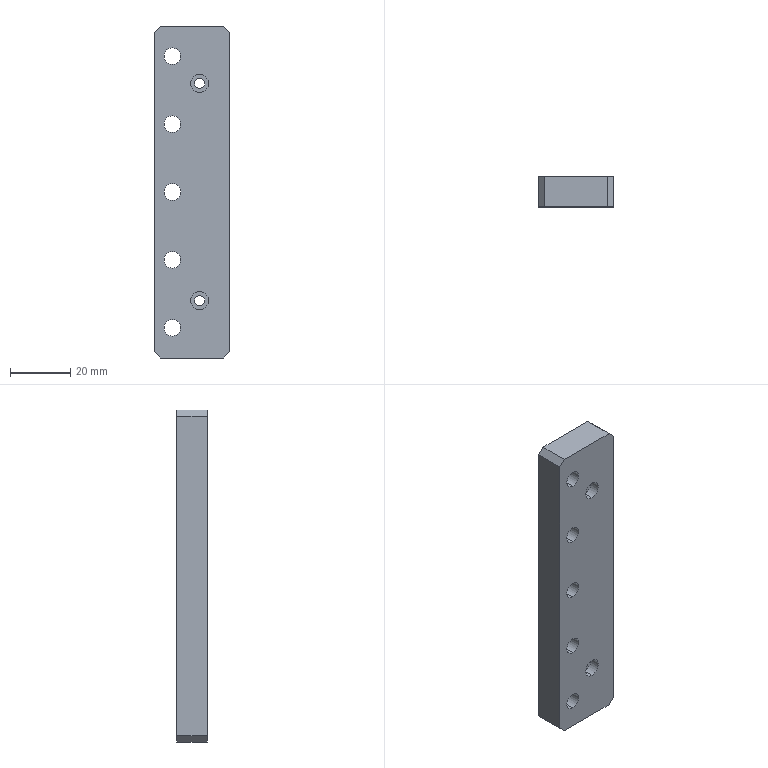Part | SolidWorks | features HoleWzd 3, Chamfer 1, Extrusion 1, ICE 1 | 1 solid | 51 faces | box 25 x 10 x 110 mm | volume 24285 mm3 | cylinder 32 | plane 19 | commonest cylinder face diameters 5.5 x10 10 x10 3.4 x4 5 x4 6 x4
STEP:
#1=CARTESIAN_POINT('',(2.5,6.5,-38.5));
#2=VERTEX_POINT('',#1);
#3=CARTESIAN_POINT('',(2.5,6.5,-33.5));
#4=VERTEX_POINT('',#3);
#5=CARTESIAN_POINT('',(2.5,6.5,-36.));
#6=DIRECTION('',(0.,1.,0.));
#7=DIRECTION('',(0.,0.,1.));
#8=AXIS2_PLACEMENT_3D('',#5,#6,#7);
#9=CIRCLE('',#8,2.5);
#10=EDGE_CURVE('',#2,#4,#9,.T.);
#11=ORIENTED_EDGE('',*,*,#10,.F.);
#12=CARTESIAN_POINT('',(2.5,10.,-38.5));
#13=VERTEX_POINT('',#12);
#14=CARTESIAN_POINT('',(2.5,6.5,-38.5));
#15=DIRECTION('',(0.,1.,0.));
#16=VECTOR('',#15,1000.);
#17=LINE('',#14,#16);
#18=EDGE_CURVE('',#2,#13,#17,.T.);
#19=ORIENTED_EDGE('',*,*,#18,.T.);
#20=CARTESIAN_POINT('',(2.5,10.,-33.5));
#21=VERTEX_POINT('',#20);
#22=CARTESIAN_POINT('',(2.5,10.,-36.));
#23=DIRECTION('',(0.,1.,0.));
#24=DIRECTION('',(0.,0.,1.));
#25=AXIS2_PLACEMENT_3D('',#22,#23,#24);
#26=CIRCLE('',#25,2.5);
#27=EDGE_CURVE('',#13,#21,#26,.T.);
#28=ORIENTED_EDGE('',*,*,#27,.T.);
#29=CARTESIAN_POINT('',(2.5,6.5,-33.5));
#30=DIRECTION('',(0.,1.,0.));
#31=VECTOR('',#30,1000.);
#32=LINE('',#29,#31);
#33=EDGE_CURVE('',#4,#21,#32,.T.);
#34=ORIENTED_EDGE('',*,*,#33,.F.);
#35=EDGE_LOOP('',(#11,#19,#28,#34));
#36=FACE_OUTER_BOUND('',#35,.T.);
#37=CARTESIAN_POINT('',(2.5,6.5,-36.));
#38=DIRECTION('',(0.,1.,0.));
#39=DIRECTION('',(0.,0.,1.));
#40=AXIS2_PLACEMENT_3D('',#37,#38,#39);
#41=CYLINDRICAL_SURFACE('',#40,2.5);
#42=ADVANCED_FACE('',(#36),#41,.F.);
#43=CARTESIAN_POINT('',(2.5,6.5,33.5));
#44=VERTEX_POINT('',#43);
#45=CARTESIAN_POINT('',(2.5,6.5,38.5));
#46=VERTEX_POINT('',#45);
#47=CARTESIAN_POINT('',(2.5,6.5,36.));
#48=DIRECTION('',(0.,1.,0.));
#49=DIRECTION('',(0.,0.,1.));
#50=AXIS2_PLACEMENT_3D('',#47,#48,#49);
#51=CIRCLE('',#50,2.5);
#52=EDGE_CURVE('',#44,#46,#51,.T.);
#53=ORIENTED_EDGE('',*,*,#52,.F.);
#54=CARTESIAN_POINT('',(2.5,10.,33.5));
#55=VERTEX_POINT('',#54);
#56=CARTESIAN_POINT('',(2.5,6.5,33.5));
#57=DIRECTION('',(0.,1.,0.));
#58=VECTOR('',#57,1000.);
#59=LINE('',#56,#58);
#60=EDGE_CURVE('',#44,#55,#59,.T.);
#61=ORIENTED_EDGE('',*,*,#60,.T.);
#62=CARTESIAN_POINT('',(2.5,10.,38.5));
#63=VERTEX_POINT('',#62);
#64=CARTESIAN_POINT('',(2.5,10.,36.));
#65=DIRECTION('',(0.,1.,0.));
#66=DIRECTION('',(0.,0.,1.));
#67=AXIS2_PLACEMENT_3D('',#64,#65,#66);
#68=CIRCLE('',#67,2.5);
#69=EDGE_CURVE('',#55,#63,#68,.T.);
#70=ORIENTED_EDGE('',*,*,#69,.T.);
#71=CARTESIAN_POINT('',(2.5,6.5,38.5));
#72=DIRECTION('',(0.,1.,0.));
#73=VECTOR('',#72,1000.);
#74=LINE('',#71,#73);
#75=EDGE_CURVE('',#46,#63,#74,.T.);
#76=ORIENTED_EDGE('',*,*,#75,.F.);
#77=EDGE_LOOP('',(#53,#61,#70,#76));
#78=FACE_OUTER_BOUND('',#77,.T.);
#79=CARTESIAN_POINT('',(2.5,6.5,36.));
#80=DIRECTION('',(0.,1.,0.));
#81=DIRECTION('',(0.,0.,1.));
#82=AXIS2_PLACEMENT_3D('',#79,#80,#81);
#83=CYLINDRICAL_SURFACE('',#82,2.5);
#84=ADVANCED_FACE('',(#78),#83,.F.);
#85=CARTESIAN_POINT('',(2.5,3.4,39.));
#86=VERTEX_POINT('',#85);
#87=CARTESIAN_POINT('',(2.5,3.4,33.));
#88=VERTEX_POINT('',#87);
#89=CARTESIAN_POINT('',(2.5,3.4,36.));
#90=DIRECTION('',(0.,-1.,0.));
#91=DIRECTION('',(0.,0.,-1.));
#92=AXIS2_PLACEMENT_3D('',#89,#90,#91);
#93=CIRCLE('',#92,3.);
#94=EDGE_CURVE('',#86,#88,#93,.T.);
#95=ORIENTED_EDGE('',*,*,#94,.F.);
#96=CARTESIAN_POINT('',(2.5,0.,39.));
#97=VERTEX_POINT('',#96);
#98=CARTESIAN_POINT('',(2.5,0.,39.));
#99=DIRECTION('',(0.,-1.,0.));
#100=VECTOR('',#99,1000.);
#101=LINE('',#98,#100);
#102=EDGE_CURVE('',#86,#97,#101,.T.);
#103=ORIENTED_EDGE('',*,*,#102,.T.);
#104=CARTESIAN_POINT('',(2.5,0.,33.));
#105=VERTEX_POINT('',#104);
#106=CARTESIAN_POINT('',(2.5,0.,36.));
#107=DIRECTION('',(0.,-1.,0.));
#108=DIRECTION('',(0.,0.,-1.));
#109=AXIS2_PLACEMENT_3D('',#106,#107,#108);
#110=CIRCLE('',#109,3.);
#111=EDGE_CURVE('',#97,#105,#110,.T.);
#112=ORIENTED_EDGE('',*,*,#111,.T.);
#113=CARTESIAN_POINT('',(2.5,0.,33.));
#114=DIRECTION('',(0.,-1.,0.));
#115=VECTOR('',#114,1000.);
#116=LINE('',#113,#115);
#117=EDGE_CURVE('',#88,#105,#116,.T.);
#118=ORIENTED_EDGE('',*,*,#117,.F.);
#119=EDGE_LOOP('',(#95,#103,#112,#118));
#120=FACE_OUTER_BOUND('',#119,.T.);
#121=CARTESIAN_POINT('',(2.5,0.,36.));
#122=DIRECTION('',(0.,-1.,0.));
#123=DIRECTION('',(0.,0.,-1.));
#124=AXIS2_PLACEMENT_3D('',#121,#122,#123);
#125=CYLINDRICAL_SURFACE('',#124,3.);
#126=ADVANCED_FACE('',(#120),#125,.F.);
#127=CARTESIAN_POINT('',(2.5,3.4,-33.));
#128=VERTEX_POINT('',#127);
#129=CARTESIAN_POINT('',(2.5,3.4,-39.));
#130=VERTEX_POINT('',#129);
#131=CARTESIAN_POINT('',(2.5,3.4,-36.));
#132=DIRECTION('',(0.,-1.,0.));
#133=DIRECTION('',(0.,0.,-1.));
#134=AXIS2_PLACEMENT_3D('',#131,#132,#133);
#135=CIRCLE('',#134,3.);
#136=EDGE_CURVE('',#128,#130,#135,.T.);
#137=ORIENTED_EDGE('',*,*,#136,.F.);
#138=CARTESIAN_POINT('',(2.5,0.,-33.));
#139=VERTEX_POINT('',#138);
#140=CARTESIAN_POINT('',(2.5,0.,-33.));
#141=DIRECTION('',(0.,-1.,0.));
#142=VECTOR('',#141,1000.);
#143=LINE('',#140,#142);
#144=EDGE_CURVE('',#128,#139,#143,.T.);
#145=ORIENTED_EDGE('',*,*,#144,.T.);
#146=CARTESIAN_POINT('',(2.5,0.,-39.));
#147=VERTEX_POINT('',#146);
#148=CARTESIAN_POINT('',(2.5,0.,-36.));
#149=DIRECTION('',(0.,-1.,0.));
#150=DIRECTION('',(0.,0.,-1.));
#151=AXIS2_PLACEMENT_3D('',#148,#149,#150);
#152=CIRCLE('',#151,3.);
#153=EDGE_CURVE('',#139,#147,#152,.T.);
#154=ORIENTED_EDGE('',*,*,#153,.T.);
#155=CARTESIAN_POINT('',(2.5,0.,-39.));
#156=DIRECTION('',(0.,-1.,0.));
#157=VECTOR('',#156,1000.);
#158=LINE('',#155,#157);
#159=EDGE_CURVE('',#130,#147,#158,.T.);
#160=ORIENTED_EDGE('',*,*,#159,.F.);
#161=EDGE_LOOP('',(#137,#145,#154,#160));
#162=FACE_OUTER_BOUND('',#161,.T.);
#163=CARTESIAN_POINT('',(2.5,0.,-36.));
#164=DIRECTION('',(0.,-1.,0.));
#165=DIRECTION('',(0.,0.,-1.));
#166=AXIS2_PLACEMENT_3D('',#163,#164,#165);
#167=CYLINDRICAL_SURFACE('',#166,3.);
#168=ADVANCED_FACE('',(#162),#167,.F.);
#169=CARTESIAN_POINT('',(-6.5,4.3,40.));
#170=VERTEX_POINT('',#169);
#171=CARTESIAN_POINT('',(-6.5,4.3,50.));
#172=VERTEX_POINT('',#171);
#173=CARTESIAN_POINT('',(-6.5,4.3,45.));
#174=DIRECTION('',(0.,1.,0.));
#175=DIRECTION('',(0.,0.,1.));
#176=AXIS2_PLACEMENT_3D('',#173,#174,#175);
#177=CIRCLE('',#176,5.);
#178=EDGE_CURVE('',#170,#172,#177,.T.);
#179=ORIENTED_EDGE('',*,*,#178,.F.);
#180=CARTESIAN_POINT('',(-6.5,10.,40.));
#181=VERTEX_POINT('',#180);
#182=CARTESIAN_POINT('',(-6.5,10.,40.));
#183=DIRECTION('',(0.,1.,0.));
#184=VECTOR('',#183,1000.);
#185=LINE('',#182,#184);
#186=EDGE_CURVE('',#170,#181,#185,.T.);
#187=ORIENTED_EDGE('',*,*,#186,.T.);
#188=CARTESIAN_POINT('',(-6.5,10.,50.));
#189=VERTEX_POINT('',#188);
#190=CARTESIAN_POINT('',(-6.5,10.,45.));
#191=DIRECTION('',(0.,1.,0.));
#192=DIRECTION('',(0.,0.,1.));
#193=AXIS2_PLACEMENT_3D('',#190,#191,#192);
#194=CIRCLE('',#193,5.);
#195=EDGE_CURVE('',#181,#189,#194,.T.);
#196=ORIENTED_EDGE('',*,*,#195,.T.);
#197=CARTESIAN_POINT('',(-6.5,10.,50.));
#198=DIRECTION('',(0.,1.,0.));
#199=VECTOR('',#198,1000.);
#200=LINE('',#197,#199);
#201=EDGE_CURVE('',#172,#189,#200,.T.);
#202=ORIENTED_EDGE('',*,*,#201,.F.);
#203=EDGE_LOOP('',(#179,#187,#196,#202));
#204=FACE_OUTER_BOUND('',#203,.T.);
#205=CARTESIAN_POINT('',(-6.5,10.,45.));
#206=DIRECTION('',(0.,1.,0.));
#207=DIRECTION('',(0.,0.,1.));
#208=AXIS2_PLACEMENT_3D('',#205,#206,#207);
#209=CYLINDRICAL_SURFACE('',#208,5.);
#210=ADVANCED_FACE('',(#204),#209,.F.);
#211=CARTESIAN_POINT('',(-6.5,0.,42.25));
#212=VERTEX_POINT('',#211);
#213=CARTESIAN_POINT('',(-6.5,0.,47.75));
#214=VERTEX_POINT('',#213);
#215=CARTESIAN_POINT('',(-6.5,0.,45.));
#216=DIRECTION('',(0.,1.,0.));
#217=DIRECTION('',(0.,0.,1.));
#218=AXIS2_PLACEMENT_3D('',#215,#216,#217);
#219=CIRCLE('',#218,2.75);
#220=EDGE_CURVE('',#212,#214,#219,.T.);
#221=ORIENTED_EDGE('',*,*,#220,.F.);
#222=CARTESIAN_POINT('',(-6.5,4.3,42.25));
#223=VERTEX_POINT('',#222);
#224=CARTESIAN_POINT('',(-6.5,10.,42.25));
#225=DIRECTION('',(0.,1.,0.));
#226=VECTOR('',#225,1000.);
#227=LINE('',#224,#226);
#228=EDGE_CURVE('',#212,#223,#227,.T.);
#229=ORIENTED_EDGE('',*,*,#228,.T.);
#230=CARTESIAN_POINT('',(-6.5,4.3,47.75));
#231=VERTEX_POINT('',#230);
#232=CARTESIAN_POINT('',(-6.5,4.3,45.));
#233=DIRECTION('',(0.,1.,0.));
#234=DIRECTION('',(0.,0.,1.));
#235=AXIS2_PLACEMENT_3D('',#232,#233,#234);
#236=CIRCLE('',#235,2.75);
#237=EDGE_CURVE('',#223,#231,#236,.T.);
#238=ORIENTED_EDGE('',*,*,#237,.T.);
#239=CARTESIAN_POINT('',(-6.5,10.,47.75));
#240=DIRECTION('',(0.,1.,0.));
#241=VECTOR('',#240,1000.);
#242=LINE('',#239,#241);
#243=EDGE_CURVE('',#214,#231,#242,.T.);
#244=ORIENTED_EDGE('',*,*,#243,.F.);
#245=EDGE_LOOP('',(#221,#229,#238,#244));
#246=FACE_OUTER_BOUND('',#245,.T.);
#247=CARTESIAN_POINT('',(-6.5,10.,45.));
#248=DIRECTION('',(0.,1.,0.));
#249=DIRECTION('',(0.,0.,1.));
#250=AXIS2_PLACEMENT_3D('',#247,#248,#249);
#251=CYLINDRICAL_SURFACE('',#250,2.75);
#252=ADVANCED_FACE('',(#246),#251,.F.);
#253=CARTESIAN_POINT('',(-6.5,4.3,-5.));
#254=VERTEX_POINT('',#253);
#255=CARTESIAN_POINT('',(-6.5,4.3,5.));
#256=VERTEX_POINT('',#255);
#257=CARTESIAN_POINT('',(-6.5,4.3,0.));
#258=DIRECTION('',(0.,1.,0.));
#259=DIRECTION('',(0.,0.,1.));
#260=AXIS2_PLACEMENT_3D('',#257,#258,#259);
#261=CIRCLE('',#260,5.);
#262=EDGE_CURVE('',#254,#256,#261,.T.);
#263=ORIENTED_EDGE('',*,*,#262,.F.);
#264=CARTESIAN_POINT('',(-6.5,10.,-5.));
#265=VERTEX_POINT('',#264);
#266=CARTESIAN_POINT('',(-6.5,10.,-5.));
#267=DIRECTION('',(0.,1.,0.));
#268=VECTOR('',#267,1000.);
#269=LINE('',#266,#268);
#270=EDGE_CURVE('',#254,#265,#269,.T.);
#271=ORIENTED_EDGE('',*,*,#270,.T.);
#272=CARTESIAN_POINT('',(-6.5,10.,5.));
#273=VERTEX_POINT('',#272);
#274=CARTESIAN_POINT('',(-6.5,10.,0.));
#275=DIRECTION('',(0.,1.,0.));
#276=DIRECTION('',(0.,0.,1.));
#277=AXIS2_PLACEMENT_3D('',#274,#275,#276);
#278=CIRCLE('',#277,5.);
#279=EDGE_CURVE('',#265,#273,#278,.T.);
#280=ORIENTED_EDGE('',*,*,#279,.T.);
#281=CARTESIAN_POINT('',(-6.5,10.,5.));
#282=DIRECTION('',(0.,1.,0.));
#283=VECTOR('',#282,1000.);
#284=LINE('',#281,#283);
#285=EDGE_CURVE('',#256,#273,#284,.T.);
#286=ORIENTED_EDGE('',*,*,#285,.F.);
#287=EDGE_LOOP('',(#263,#271,#280,#286));
#288=FACE_OUTER_BOUND('',#287,.T.);
#289=CARTESIAN_POINT('',(-6.5,10.,0.));
#290=DIRECTION('',(0.,1.,0.));
#291=DIRECTION('',(0.,0.,1.));
#292=AXIS2_PLACEMENT_3D('',#289,#290,#291);
#293=CYLINDRICAL_SURFACE('',#292,5.);
#294=ADVANCED_FACE('',(#288),#293,.F.);
#295=CARTESIAN_POINT('',(-6.5,0.,-2.75));
#296=VERTEX_POINT('',#295);
#297=CARTESIAN_POINT('',(-6.5,0.,2.75));
#298=VERTEX_POINT('',#297);
#299=CARTESIAN_POINT('',(-6.5,0.,0.));
#300=DIRECTION('',(0.,1.,0.));
#301=DIRECTION('',(0.,0.,1.));
#302=AXIS2_PLACEMENT_3D('',#299,#300,#301);
#303=CIRCLE('',#302,2.75);
#304=EDGE_CURVE('',#296,#298,#303,.T.);
#305=ORIENTED_EDGE('',*,*,#304,.F.);
#306=CARTESIAN_POINT('',(-6.5,4.3,-2.75));
#307=VERTEX_POINT('',#306);
#308=CARTESIAN_POINT('',(-6.5,10.,-2.75));
#309=DIRECTION('',(0.,1.,0.));
#310=VECTOR('',#309,1000.);
#311=LINE('',#308,#310);
#312=EDGE_CURVE('',#296,#307,#311,.T.);
#313=ORIENTED_EDGE('',*,*,#312,.T.);
#314=CARTESIAN_POINT('',(-6.5,4.3,2.75));
#315=VERTEX_POINT('',#314);
#316=CARTESIAN_POINT('',(-6.5,4.3,0.));
#317=DIRECTION('',(0.,1.,0.));
#318=DIRECTION('',(0.,0.,1.));
#319=AXIS2_PLACEMENT_3D('',#316,#317,#318);
#320=CIRCLE('',#319,2.75);
#321=EDGE_CURVE('',#307,#315,#320,.T.);
#322=ORIENTED_EDGE('',*,*,#321,.T.);
#323=CARTESIAN_POINT('',(-6.5,10.,2.75));
#324=DIRECTION('',(0.,1.,0.));
#325=VECTOR('',#324,1000.);
#326=LINE('',#323,#325);
#327=EDGE_CURVE('',#298,#315,#326,.T.);
#328=ORIENTED_EDGE('',*,*,#327,.F.);
#329=EDGE_LOOP('',(#305,#313,#322,#328));
#330=FACE_OUTER_BOUND('',#329,.T.);
#331=CARTESIAN_POINT('',(-6.5,10.,0.));
#332=DIRECTION('',(0.,1.,0.));
#333=DIRECTION('',(0.,0.,1.));
#334=AXIS2_PLACEMENT_3D('',#331,#332,#333);
#335=CYLINDRICAL_SURFACE('',#334,2.75);
#336=ADVANCED_FACE('',(#330),#335,.F.);
#337=CARTESIAN_POINT('',(-6.5,4.3,-50.));
#338=VERTEX_POINT('',#337);
#339=CARTESIAN_POINT('',(-6.5,4.3,-40.));
#340=VERTEX_POINT('',#339);
#341=CARTESIAN_POINT('',(-6.5,4.3,-45.));
#342=DIRECTION('',(0.,1.,0.));
#343=DIRECTION('',(0.,0.,1.));
#344=AXIS2_PLACEMENT_3D('',#341,#342,#343);
#345=CIRCLE('',#344,5.);
#346=EDGE_CURVE('',#338,#340,#345,.T.);
#347=ORIENTED_EDGE('',*,*,#346,.F.);
#348=CARTESIAN_POINT('',(-6.5,10.,-50.));
#349=VERTEX_POINT('',#348);
#350=CARTESIAN_POINT('',(-6.5,10.,-50.));
#351=DIRECTION('',(0.,1.,0.));
#352=VECTOR('',#351,1000.);
#353=LINE('',#350,#352);
#354=EDGE_CURVE('',#338,#349,#353,.T.);
#355=ORIENTED_EDGE('',*,*,#354,.T.);
#356=CARTESIAN_POINT('',(-6.5,10.,-40.));
#357=VERTEX_POINT('',#356);
#358=CARTESIAN_POINT('',(-6.5,10.,-45.));
#359=DIRECTION('',(0.,1.,0.));
#360=DIRECTION('',(0.,0.,1.));
#361=AXIS2_PLACEMENT_3D('',#358,#359,#360);
#362=CIRCLE('',#361,5.);
#363=EDGE_CURVE('',#349,#357,#362,.T.);
#364=ORIENTED_EDGE('',*,*,#363,.T.);
#365=CARTESIAN_POINT('',(-6.5,10.,-40.));
#366=DIRECTION('',(0.,1.,0.));
#367=VECTOR('',#366,1000.);
#368=LINE('',#365,#367);
#369=EDGE_CURVE('',#340,#357,#368,.T.);
#370=ORIENTED_EDGE('',*,*,#369,.F.);
#371=EDGE_LOOP('',(#347,#355,#364,#370));
#372=FACE_OUTER_BOUND('',#371,.T.);
#373=CARTESIAN_POINT('',(-6.5,10.,-45.));
#374=DIRECTION('',(0.,1.,0.));
#375=DIRECTION('',(0.,0.,1.));
#376=AXIS2_PLACEMENT_3D('',#373,#374,#375);
#377=CYLINDRICAL_SURFACE('',#376,5.);
#378=ADVANCED_FACE('',(#372),#377,.F.);
#379=CARTESIAN_POINT('',(-6.5,0.,-47.75));
#380=VERTEX_POINT('',#379);
#381=CARTESIAN_POINT('',(-6.5,0.,-42.25));
#382=VERTEX_POINT('',#381);
#383=CARTESIAN_POINT('',(-6.5,0.,-45.));
#384=DIRECTION('',(0.,1.,0.));
#385=DIRECTION('',(0.,0.,1.));
#386=AXIS2_PLACEMENT_3D('',#383,#384,#385);
#387=CIRCLE('',#386,2.75);
#388=EDGE_CURVE('',#380,#382,#387,.T.);
#389=ORIENTED_EDGE('',*,*,#388,.F.);
#390=CARTESIAN_POINT('',(-6.5,4.3,-47.75));
#391=VERTEX_POINT('',#390);
#392=CARTESIAN_POINT('',(-6.5,10.,-47.75));
#393=DIRECTION('',(0.,1.,0.));
#394=VECTOR('',#393,1000.);
#395=LINE('',#392,#394);
#396=EDGE_CURVE('',#380,#391,#395,.T.);
#397=ORIENTED_EDGE('',*,*,#396,.T.);
#398=CARTESIAN_POINT('',(-6.5,4.3,-42.25));
#399=VERTEX_POINT('',#398);
#400=CARTESIAN_POINT('',(-6.5,4.3,-45.));
#401=DIRECTION('',(0.,1.,0.));
#402=DIRECTION('',(0.,0.,1.));
#403=AXIS2_PLACEMENT_3D('',#400,#401,#402);
#404=CIRCLE('',#403,2.75);
#405=EDGE_CURVE('',#391,#399,#404,.T.);
#406=ORIENTED_EDGE('',*,*,#405,.T.);
#407=CARTESIAN_POINT('',(-6.5,10.,-42.25));
#408=DIRECTION('',(0.,1.,0.));
#409=VECTOR('',#408,1000.);
#410=LINE('',#407,#409);
#411=EDGE_CURVE('',#382,#399,#410,.T.);
#412=ORIENTED_EDGE('',*,*,#411,.F.);
#413=EDGE_LOOP('',(#389,#397,#406,#412));
#414=FACE_OUTER_BOUND('',#413,.T.);
#415=CARTESIAN_POINT('',(-6.5,10.,-45.));
#416=DIRECTION('',(0.,1.,0.));
#417=DIRECTION('',(0.,0.,1.));
#418=AXIS2_PLACEMENT_3D('',#415,#416,#417);
#419=CYLINDRICAL_SURFACE('',#418,2.75);
#420=ADVANCED_FACE('',(#414),#419,.F.);
#421=CARTESIAN_POINT('',(-6.5,4.3,17.5));
#422=VERTEX_POINT('',#421);
#423=CARTESIAN_POINT('',(-6.5,4.3,27.5));
#424=VERTEX_POINT('',#423);
#425=CARTESIAN_POINT('',(-6.5,4.3,22.5));
#426=DIRECTION('',(0.,1.,0.));
#427=DIRECTION('',(0.,0.,1.));
#428=AXIS2_PLACEMENT_3D('',#425,#426,#427);
#429=CIRCLE('',#428,5.);
#430=EDGE_CURVE('',#422,#424,#429,.T.);
#431=ORIENTED_EDGE('',*,*,#430,.F.);
#432=CARTESIAN_POINT('',(-6.5,10.,17.5));
#433=VERTEX_POINT('',#432);
#434=CARTESIAN_POINT('',(-6.5,10.,17.5));
#435=DIRECTION('',(0.,1.,0.));
#436=VECTOR('',#435,1000.);
#437=LINE('',#434,#436);
#438=EDGE_CURVE('',#422,#433,#437,.T.);
#439=ORIENTED_EDGE('',*,*,#438,.T.);
#440=CARTESIAN_POINT('',(-6.5,10.,27.5));
#441=VERTEX_POINT('',#440);
#442=CARTESIAN_POINT('',(-6.5,10.,22.5));
#443=DIRECTION('',(0.,1.,0.));
#444=DIRECTION('',(0.,0.,1.));
#445=AXIS2_PLACEMENT_3D('',#442,#443,#444);
#446=CIRCLE('',#445,5.);
#447=EDGE_CURVE('',#433,#441,#446,.T.);
#448=ORIENTED_EDGE('',*,*,#447,.T.);
#449=CARTESIAN_POINT('',(-6.5,10.,27.5));
#450=DIRECTION('',(0.,1.,0.));
#451=VECTOR('',#450,1000.);
#452=LINE('',#449,#451);
#453=EDGE_CURVE('',#424,#441,#452,.T.);
#454=ORIENTED_EDGE('',*,*,#453,.F.);
#455=EDGE_LOOP('',(#431,#439,#448,#454));
#456=FACE_OUTER_BOUND('',#455,.T.);
#457=CARTESIAN_POINT('',(-6.5,10.,22.5));
#458=DIRECTION('',(0.,1.,0.));
#459=DIRECTION('',(0.,0.,1.));
#460=AXIS2_PLACEMENT_3D('',#457,#458,#459);
#461=CYLINDRICAL_SURFACE('',#460,5.);
#462=ADVANCED_FACE('',(#456),#461,.F.);
#463=CARTESIAN_POINT('',(-6.5,0.,19.75));
#464=VERTEX_POINT('',#463);
#465=CARTESIAN_POINT('',(-6.5,0.,25.25));
#466=VERTEX_POINT('',#465);
#467=CARTESIAN_POINT('',(-6.5,0.,22.5));
#468=DIRECTION('',(0.,1.,0.));
#469=DIRECTION('',(0.,0.,1.));
#470=AXIS2_PLACEMENT_3D('',#467,#468,#469);
#471=CIRCLE('',#470,2.75);
#472=EDGE_CURVE('',#464,#466,#471,.T.);
#473=ORIENTED_EDGE('',*,*,#472,.F.);
#474=CARTESIAN_POINT('',(-6.5,4.3,19.75));
#475=VERTEX_POINT('',#474);
#476=CARTESIAN_POINT('',(-6.5,10.,19.75));
#477=DIRECTION('',(0.,1.,0.));
#478=VECTOR('',#477,1000.);
#479=LINE('',#476,#478);
#480=EDGE_CURVE('',#464,#475,#479,.T.);
#481=ORIENTED_EDGE('',*,*,#480,.T.);
#482=CARTESIAN_POINT('',(-6.5,4.3,25.25));
#483=VERTEX_POINT('',#482);
#484=CARTESIAN_POINT('',(-6.5,4.3,22.5));
#485=DIRECTION('',(0.,1.,0.));
#486=DIRECTION('',(0.,0.,1.));
#487=AXIS2_PLACEMENT_3D('',#484,#485,#486);
#488=CIRCLE('',#487,2.75);
#489=EDGE_CURVE('',#475,#483,#488,.T.);
#490=ORIENTED_EDGE('',*,*,#489,.T.);
#491=CARTESIAN_POINT('',(-6.5,10.,25.25));
#492=DIRECTION('',(0.,1.,0.));
#493=VECTOR('',#492,1000.);
#494=LINE('',#491,#493);
#495=EDGE_CURVE('',#466,#483,#494,.T.);
#496=ORIENTED_EDGE('',*,*,#495,.F.);
#497=EDGE_LOOP('',(#473,#481,#490,#496));
#498=FACE_OUTER_BOUND('',#497,.T.);
#499=CARTESIAN_POINT('',(-6.5,10.,22.5));
#500=DIRECTION('',(0.,1.,0.));
#501=DIRECTION('',(0.,0.,1.));
#502=AXIS2_PLACEMENT_3D('',#499,#500,#501);
#503=CYLINDRICAL_SURFACE('',#502,2.75);
#504=ADVANCED_FACE('',(#498),#503,.F.);
#505=CARTESIAN_POINT('',(-6.5,4.3,-27.5));
#506=VERTEX_POINT('',#505);
#507=CARTESIAN_POINT('',(-6.5,4.3,-17.5));
#508=VERTEX_POINT('',#507);
#509=CARTESIAN_POINT('',(-6.5,4.3,-22.5));
#510=DIRECTION('',(0.,1.,0.));
#511=DIRECTION('',(0.,0.,1.));
#512=AXIS2_PLACEMENT_3D('',#509,#510,#511);
#513=CIRCLE('',#512,5.);
#514=EDGE_CURVE('',#506,#508,#513,.T.);
#515=ORIENTED_EDGE('',*,*,#514,.F.);
#516=CARTESIAN_POINT('',(-6.5,10.,-27.5));
#517=VERTEX_POINT('',#516);
#518=CARTESIAN_POINT('',(-6.5,10.,-27.5));
#519=DIRECTION('',(0.,1.,0.));
#520=VECTOR('',#519,1000.);
#521=LINE('',#518,#520);
#522=EDGE_CURVE('',#506,#517,#521,.T.);
#523=ORIENTED_EDGE('',*,*,#522,.T.);
#524=CARTESIAN_POINT('',(-6.5,10.,-17.5));
#525=VERTEX_POINT('',#524);
#526=CARTESIAN_POINT('',(-6.5,10.,-22.5));
#527=DIRECTION('',(0.,1.,0.));
#528=DIRECTION('',(0.,0.,1.));
#529=AXIS2_PLACEMENT_3D('',#526,#527,#528);
#530=CIRCLE('',#529,5.);
#531=EDGE_CURVE('',#517,#525,#530,.T.);
#532=ORIENTED_EDGE('',*,*,#531,.T.);
#533=CARTESIAN_POINT('',(-6.5,10.,-17.5));
#534=DIRECTION('',(0.,1.,0.));
#535=VECTOR('',#534,1000.);
#536=LINE('',#533,#535);
#537=EDGE_CURVE('',#508,#525,#536,.T.);
#538=ORIENTED_EDGE('',*,*,#537,.F.);
#539=EDGE_LOOP('',(#515,#523,#532,#538));
#540=FACE_OUTER_BOUND('',#539,.T.);
#541=CARTESIAN_POINT('',(-6.5,10.,-22.5));
#542=DIRECTION('',(0.,1.,0.));
#543=DIRECTION('',(0.,0.,1.));
#544=AXIS2_PLACEMENT_3D('',#541,#542,#543);
#545=CYLINDRICAL_SURFACE('',#544,5.);
#546=ADVANCED_FACE('',(#540),#545,.F.);
#547=CARTESIAN_POINT('',(-6.5,0.,-25.25));
#548=VERTEX_POINT('',#547);
#549=CARTESIAN_POINT('',(-6.5,0.,-19.75));
#550=VERTEX_POINT('',#549);
#551=CARTESIAN_POINT('',(-6.5,0.,-22.5));
#552=DIRECTION('',(0.,1.,0.));
#553=DIRECTION('',(0.,0.,1.));
#554=AXIS2_PLACEMENT_3D('',#551,#552,#553);
#555=CIRCLE('',#554,2.75);
#556=EDGE_CURVE('',#548,#550,#555,.T.);
#557=ORIENTED_EDGE('',*,*,#556,.F.);
#558=CARTESIAN_POINT('',(-6.5,4.3,-25.25));
#559=VERTEX_POINT('',#558);
#560=CARTESIAN_POINT('',(-6.5,10.,-25.25));
#561=DIRECTION('',(0.,1.,0.));
#562=VECTOR('',#561,1000.);
#563=LINE('',#560,#562);
#564=EDGE_CURVE('',#548,#559,#563,.T.);
#565=ORIENTED_EDGE('',*,*,#564,.T.);
#566=CARTESIAN_POINT('',(-6.5,4.3,-19.75));
#567=VERTEX_POINT('',#566);
#568=CARTESIAN_POINT('',(-6.5,4.3,-22.5));
#569=DIRECTION('',(0.,1.,0.));
#570=DIRECTION('',(0.,0.,1.));
#571=AXIS2_PLACEMENT_3D('',#568,#569,#570);
#572=CIRCLE('',#571,2.75);
#573=EDGE_CURVE('',#559,#567,#572,.T.);
#574=ORIENTED_EDGE('',*,*,#573,.T.);
#575=CARTESIAN_POINT('',(-6.5,10.,-19.75));
#576=DIRECTION('',(0.,1.,0.));
#577=VECTOR('',#576,1000.);
#578=LINE('',#575,#577);
#579=EDGE_CURVE('',#550,#567,#578,.T.);
#580=ORIENTED_EDGE('',*,*,#579,.F.);
#581=EDGE_LOOP('',(#557,#565,#574,#580));
#582=FACE_OUTER_BOUND('',#581,.T.);
#583=CARTESIAN_POINT('',(-6.5,10.,-22.5));
#584=DIRECTION('',(0.,1.,0.));
#585=DIRECTION('',(0.,0.,1.));
#586=AXIS2_PLACEMENT_3D('',#583,#584,#585);
#587=CYLINDRICAL_SURFACE('',#586,2.75);
#588=ADVANCED_FACE('',(#582),#587,.F.);
#589=CARTESIAN_POINT('',(2.5,6.5,37.7));
#590=VERTEX_POINT('',#589);
#591=CARTESIAN_POINT('',(2.5,6.5,34.3));
#592=VERTEX_POINT('',#591);
#593=CARTESIAN_POINT('',(2.5,6.5,36.));
#594=DIRECTION('',(0.,-1.,0.));
#595=DIRECTION('',(0.,0.,1.));
#596=AXIS2_PLACEMENT_3D('',#593,#594,#595);
#597=CIRCLE('',#596,1.7);
#598=EDGE_CURVE('',#590,#592,#597,.T.);
#599=ORIENTED_EDGE('',*,*,#598,.F.);
#600=CARTESIAN_POINT('',(2.5,3.4,37.7));
#601=VERTEX_POINT('',#600);
#602=CARTESIAN_POINT('',(2.5,0.,37.7));
#603=DIRECTION('',(0.,-1.,0.));
#604=VECTOR('',#603,1000.);
#605=LINE('',#602,#604);
#606=EDGE_CURVE('',#590,#601,#605,.T.);
#607=ORIENTED_EDGE('',*,*,#606,.T.);
#608=CARTESIAN_POINT('',(2.5,3.4,34.3));
#609=VERTEX_POINT('',#608);
#610=CARTESIAN_POINT('',(2.5,3.4,36.));
#611=DIRECTION('',(0.,-1.,0.));
#612=DIRECTION('',(0.,0.,-1.));
#613=AXIS2_PLACEMENT_3D('',#610,#611,#612);
#614=CIRCLE('',#613,1.7);
#615=EDGE_CURVE('',#601,#609,#614,.T.);
#616=ORIENTED_EDGE('',*,*,#615,.T.);
#617=CARTESIAN_POINT('',(2.5,0.,34.3));
#618=DIRECTION('',(0.,-1.,0.));
#619=VECTOR('',#618,1000.);
#620=LINE('',#617,#619);
#621=EDGE_CURVE('',#592,#609,#620,.T.);
#622=ORIENTED_EDGE('',*,*,#621,.F.);
#623=EDGE_LOOP('',(#599,#607,#616,#622));
#624=FACE_OUTER_BOUND('',#623,.T.);
#625=CARTESIAN_POINT('',(2.5,0.,36.));
#626=DIRECTION('',(0.,-1.,0.));
#627=DIRECTION('',(0.,0.,-1.));
#628=AXIS2_PLACEMENT_3D('',#625,#626,#627);
#629=CYLINDRICAL_SURFACE('',#628,1.7);
#630=ADVANCED_FACE('',(#624),#629,.F.);
#631=CARTESIAN_POINT('',(2.5,6.5,-34.3));
#632=VERTEX_POINT('',#631);
#633=CARTESIAN_POINT('',(2.5,6.5,-37.7));
#634=VERTEX_POINT('',#633);
#635=CARTESIAN_POINT('',(2.5,6.5,-36.));
#636=DIRECTION('',(0.,-1.,0.));
#637=DIRECTION('',(0.,0.,1.));
#638=AXIS2_PLACEMENT_3D('',#635,#636,#637);
#639=CIRCLE('',#638,1.7);
#640=EDGE_CURVE('',#632,#634,#639,.T.);
#641=ORIENTED_EDGE('',*,*,#640,.F.);
#642=CARTESIAN_POINT('',(2.5,3.4,-34.3));
#643=VERTEX_POINT('',#642);
#644=CARTESIAN_POINT('',(2.5,0.,-34.3));
#645=DIRECTION('',(0.,-1.,0.));
#646=VECTOR('',#645,1000.);
#647=LINE('',#644,#646);
#648=EDGE_CURVE('',#632,#643,#647,.T.);
#649=ORIENTED_EDGE('',*,*,#648,.T.);
#650=CARTESIAN_POINT('',(2.5,3.4,-37.7));
#651=VERTEX_POINT('',#650);
#652=CARTESIAN_POINT('',(2.5,3.4,-36.));
#653=DIRECTION('',(0.,-1.,0.));
#654=DIRECTION('',(0.,0.,-1.));
#655=AXIS2_PLACEMENT_3D('',#652,#653,#654);
#656=CIRCLE('',#655,1.7);
#657=EDGE_CURVE('',#643,#651,#656,.T.);
#658=ORIENTED_EDGE('',*,*,#657,.T.);
#659=CARTESIAN_POINT('',(2.5,0.,-37.7));
#660=DIRECTION('',(0.,-1.,0.));
#661=VECTOR('',#660,1000.);
#662=LINE('',#659,#661);
#663=EDGE_CURVE('',#634,#651,#662,.T.);
#664=ORIENTED_EDGE('',*,*,#663,.F.);
#665=EDGE_LOOP('',(#641,#649,#658,#664));
#666=FACE_OUTER_BOUND('',#665,.T.);
#667=CARTESIAN_POINT('',(2.5,0.,-36.));
#668=DIRECTION('',(0.,-1.,0.));
#669=DIRECTION('',(0.,0.,-1.));
#670=AXIS2_PLACEMENT_3D('',#667,#668,#669);
#671=CYLINDRICAL_SURFACE('',#670,1.7);
#672=ADVANCED_FACE('',(#666),#671,.F.);
#673=ORIENTED_EDGE('',*,*,#648,.F.);
#674=CARTESIAN_POINT('',(2.5,6.5,-36.));
#675=DIRECTION('',(0.,-1.,0.));
#676=DIRECTION('',(0.,0.,1.));
#677=AXIS2_PLACEMENT_3D('',#674,#675,#676);
#678=CIRCLE('',#677,1.7);
#679=EDGE_CURVE('',#634,#632,#678,.T.);
#680=ORIENTED_EDGE('',*,*,#679,.F.);
#681=ORIENTED_EDGE('',*,*,#663,.T.);
#682=CARTESIAN_POINT('',(2.5,3.4,-36.));
#683=DIRECTION('',(0.,-1.,0.));
#684=DIRECTION('',(0.,0.,-1.));
#685=AXIS2_PLACEMENT_3D('',#682,#683,#684);
#686=CIRCLE('',#685,1.7);
#687=EDGE_CURVE('',#651,#643,#686,.T.);
#688=ORIENTED_EDGE('',*,*,#687,.T.);
#689=EDGE_LOOP('',(#673,#680,#681,#688));
#690=FACE_OUTER_BOUND('',#689,.T.);
#691=CARTESIAN_POINT('',(2.5,0.,-36.));
#692=DIRECTION('',(0.,-1.,0.));
#693=DIRECTION('',(0.,0.,-1.));
#694=AXIS2_PLACEMENT_3D('',#691,#692,#693);
#695=CYLINDRICAL_SURFACE('',#694,1.7);
#696=ADVANCED_FACE('',(#690),#695,.F.);
#697=ORIENTED_EDGE('',*,*,#606,.F.);
#698=CARTESIAN_POINT('',(2.5,6.5,36.));
#699=DIRECTION('',(0.,-1.,0.));
#700=DIRECTION('',(0.,0.,1.));
#701=AXIS2_PLACEMENT_3D('',#698,#699,#700);
#702=CIRCLE('',#701,1.7);
#703=EDGE_CURVE('',#592,#590,#702,.T.);
#704=ORIENTED_EDGE('',*,*,#703,.F.);
#705=ORIENTED_EDGE('',*,*,#621,.T.);
#706=CARTESIAN_POINT('',(2.5,3.4,36.));
#707=DIRECTION('',(0.,-1.,0.));
#708=DIRECTION('',(0.,0.,-1.));
#709=AXIS2_PLACEMENT_3D('',#706,#707,#708);
#710=CIRCLE('',#709,1.7);
#711=EDGE_CURVE('',#609,#601,#710,.T.);
#712=ORIENTED_EDGE('',*,*,#711,.T.);
#713=EDGE_LOOP('',(#697,#704,#705,#712));
#714=FACE_OUTER_BOUND('',#713,.T.);
#715=CARTESIAN_POINT('',(2.5,0.,36.));
#716=DIRECTION('',(0.,-1.,0.));
#717=DIRECTION('',(0.,0.,-1.));
#718=AXIS2_PLACEMENT_3D('',#715,#716,#717);
#719=CYLINDRICAL_SURFACE('',#718,1.7);
#720=ADVANCED_FACE('',(#714),#719,.F.);
#721=CARTESIAN_POINT('',(12.5,0.,53.));
#722=VERTEX_POINT('',#721);
#723=CARTESIAN_POINT('',(12.5,0.,-53.));
#724=VERTEX_POINT('',#723);
#725=CARTESIAN_POINT('',(12.5,0.,-55.));
#726=DIRECTION('',(0.,0.,-1.));
#727=VECTOR('',#726,1000.);
#728=LINE('',#725,#727);
#729=EDGE_CURVE('',#722,#724,#728,.T.);
#730=ORIENTED_EDGE('',*,*,#729,.T.);
#731=CARTESIAN_POINT('',(12.5,10.,-53.));
#732=VERTEX_POINT('',#731);
#733=CARTESIAN_POINT('',(12.5,10.,-53.));
#734=DIRECTION('',(0.,1.,0.));
#735=VECTOR('',#734,1000.);
#736=LINE('',#733,#735);
#737=EDGE_CURVE('',#724,#732,#736,.T.);
#738=ORIENTED_EDGE('',*,*,#737,.T.);
#739=CARTESIAN_POINT('',(12.5,10.,53.));
#740=VERTEX_POINT('',#739);
#741=CARTESIAN_POINT('',(12.5,10.,-55.));
#742=DIRECTION('',(0.,0.,-1.));
#743=VECTOR('',#742,1000.);
#744=LINE('',#741,#743);
#745=EDGE_CURVE('',#740,#732,#744,.T.);
#746=ORIENTED_EDGE('',*,*,#745,.F.);
#747=CARTESIAN_POINT('',(12.5,10.,53.));
#748=DIRECTION('',(0.,-1.,0.));
#749=VECTOR('',#748,1000.);
#750=LINE('',#747,#749);
#751=EDGE_CURVE('',#740,#722,#750,.T.);
#752=ORIENTED_EDGE('',*,*,#751,.T.);
#753=EDGE_LOOP('',(#730,#738,#746,#752));
#754=FACE_OUTER_BOUND('',#753,.T.);
#755=CARTESIAN_POINT('',(12.5,10.,-55.));
#756=DIRECTION('',(-1.,0.,0.));
#757=DIRECTION('',(0.,0.,1.));
#758=AXIS2_PLACEMENT_3D('',#755,#756,#757);
#759=PLANE('',#758);
#760=ADVANCED_FACE('',(#754),#759,.F.);
#761=CARTESIAN_POINT('',(10.5,0.,-55.));
#762=VERTEX_POINT('',#761);
#763=CARTESIAN_POINT('',(-10.5,0.,-55.));
#764=VERTEX_POINT('',#763);
#765=CARTESIAN_POINT('',(-12.5,0.,-55.));
#766=DIRECTION('',(-1.,0.,0.));
#767=VECTOR('',#766,1000.);
#768=LINE('',#765,#767);
#769=EDGE_CURVE('',#762,#764,#768,.T.);
#770=ORIENTED_EDGE('',*,*,#769,.T.);
#771=CARTESIAN_POINT('',(-10.5,10.,-55.));
#772=VERTEX_POINT('',#771);
#773=CARTESIAN_POINT('',(-10.5,10.,-55.));
#774=DIRECTION('',(0.,1.,0.));
#775=VECTOR('',#774,1000.);
#776=LINE('',#773,#775);
#777=EDGE_CURVE('',#764,#772,#776,.T.);
#778=ORIENTED_EDGE('',*,*,#777,.T.);
#779=CARTESIAN_POINT('',(10.5,10.,-55.));
#780=VERTEX_POINT('',#779);
#781=CARTESIAN_POINT('',(-12.5,10.,-55.));
#782=DIRECTION('',(-1.,0.,0.));
#783=VECTOR('',#782,1000.);
#784=LINE('',#781,#783);
#785=EDGE_CURVE('',#780,#772,#784,.T.);
#786=ORIENTED_EDGE('',*,*,#785,.F.);
#787=CARTESIAN_POINT('',(10.5,10.,-55.));
#788=DIRECTION('',(0.,-1.,0.));
#789=VECTOR('',#788,1000.);
#790=LINE('',#787,#789);
#791=EDGE_CURVE('',#780,#762,#790,.T.);
#792=ORIENTED_EDGE('',*,*,#791,.T.);
#793=EDGE_LOOP('',(#770,#778,#786,#792));
#794=FACE_OUTER_BOUND('',#793,.T.);
#795=CARTESIAN_POINT('',(-12.5,10.,-55.));
#796=DIRECTION('',(0.,0.,1.));
#797=DIRECTION('',(1.,0.,0.));
#798=AXIS2_PLACEMENT_3D('',#795,#796,#797);
#799=PLANE('',#798);
#800=ADVANCED_FACE('',(#794),#799,.F.);
#801=CARTESIAN_POINT('',(-12.5,10.,-53.));
#802=VERTEX_POINT('',#801);
#803=CARTESIAN_POINT('',(-12.5,10.,53.));
#804=VERTEX_POINT('',#803);
#805=CARTESIAN_POINT('',(-12.5,10.,-55.));
#806=DIRECTION('',(0.,0.,1.));
#807=VECTOR('',#806,1000.);
#808=LINE('',#805,#807);
#809=EDGE_CURVE('',#802,#804,#808,.T.);
#810=ORIENTED_EDGE('',*,*,#809,.F.);
#811=CARTESIAN_POINT('',(-12.5,0.,-53.));
#812=VERTEX_POINT('',#811);
#813=CARTESIAN_POINT('',(-12.5,10.,-53.));
#814=DIRECTION('',(0.,-1.,0.));
#815=VECTOR('',#814,1000.);
#816=LINE('',#813,#815);
#817=EDGE_CURVE('',#802,#812,#816,.T.);
#818=ORIENTED_EDGE('',*,*,#817,.T.);
#819=CARTESIAN_POINT('',(-12.5,0.,53.));
#820=VERTEX_POINT('',#819);
#821=CARTESIAN_POINT('',(-12.5,0.,-55.));
#822=DIRECTION('',(0.,0.,1.));
#823=VECTOR('',#822,1000.);
#824=LINE('',#821,#823);
#825=EDGE_CURVE('',#812,#820,#824,.T.);
#826=ORIENTED_EDGE('',*,*,#825,.T.);
#827=CARTESIAN_POINT('',(-12.5,10.,53.));
#828=DIRECTION('',(0.,1.,0.));
#829=VECTOR('',#828,1000.);
#830=LINE('',#827,#829);
#831=EDGE_CURVE('',#820,#804,#830,.T.);
#832=ORIENTED_EDGE('',*,*,#831,.T.);
#833=EDGE_LOOP('',(#810,#818,#826,#832));
#834=FACE_OUTER_BOUND('',#833,.T.);
#835=CARTESIAN_POINT('',(-12.5,10.,-55.));
#836=DIRECTION('',(1.,0.,0.));
#837=DIRECTION('',(0.,0.,-1.));
#838=AXIS2_PLACEMENT_3D('',#835,#836,#837);
#839=PLANE('',#838);
#840=ADVANCED_FACE('',(#834),#839,.F.);
#841=CARTESIAN_POINT('',(-10.5,10.,55.));
#842=VERTEX_POINT('',#841);
#843=CARTESIAN_POINT('',(10.5,10.,55.));
#844=VERTEX_POINT('',#843);
#845=CARTESIAN_POINT('',(-12.5,10.,55.));
#846=DIRECTION('',(1.,0.,0.));
#847=VECTOR('',#846,1000.);
#848=LINE('',#845,#847);
#849=EDGE_CURVE('',#842,#844,#848,.T.);
#850=ORIENTED_EDGE('',*,*,#849,.F.);
#851=CARTESIAN_POINT('',(-10.5,0.,55.));
#852=VERTEX_POINT('',#851);
#853=CARTESIAN_POINT('',(-10.5,10.,55.));
#854=DIRECTION('',(0.,-1.,0.));
#855=VECTOR('',#854,1000.);
#856=LINE('',#853,#855);
#857=EDGE_CURVE('',#842,#852,#856,.T.);
#858=ORIENTED_EDGE('',*,*,#857,.T.);
#859=CARTESIAN_POINT('',(10.5,0.,55.));
#860=VERTEX_POINT('',#859);
#861=CARTESIAN_POINT('',(-12.5,0.,55.));
#862=DIRECTION('',(1.,0.,0.));
#863=VECTOR('',#862,1000.);
#864=LINE('',#861,#863);
#865=EDGE_CURVE('',#852,#860,#864,.T.);
#866=ORIENTED_EDGE('',*,*,#865,.T.);
#867=CARTESIAN_POINT('',(10.5,10.,55.));
#868=DIRECTION('',(0.,1.,0.));
#869=VECTOR('',#868,1000.);
#870=LINE('',#867,#869);
#871=EDGE_CURVE('',#860,#844,#870,.T.);
#872=ORIENTED_EDGE('',*,*,#871,.T.);
#873=EDGE_LOOP('',(#850,#858,#866,#872));
#874=FACE_OUTER_BOUND('',#873,.T.);
#875=CARTESIAN_POINT('',(-12.5,10.,55.));
#876=DIRECTION('',(0.,0.,-1.));
#877=DIRECTION('',(-1.,0.,0.));
#878=AXIS2_PLACEMENT_3D('',#875,#876,#877);
#879=PLANE('',#878);
#880=ADVANCED_FACE('',(#874),#879,.F.);
#881=CARTESIAN_POINT('',(2.5,10.,36.));
#882=DIRECTION('',(0.,1.,0.));
#883=DIRECTION('',(0.,0.,1.));
#884=AXIS2_PLACEMENT_3D('',#881,#882,#883);
#885=CIRCLE('',#884,2.5);
#886=EDGE_CURVE('',#63,#55,#885,.T.);
#887=ORIENTED_EDGE('',*,*,#886,.F.);
#888=ORIENTED_EDGE('',*,*,#69,.F.);
#889=EDGE_LOOP('',(#887,#888));
#890=FACE_BOUND('',#889,.T.);
#891=CARTESIAN_POINT('',(2.5,10.,-36.));
#892=DIRECTION('',(0.,1.,0.));
#893=DIRECTION('',(0.,0.,1.));
#894=AXIS2_PLACEMENT_3D('',#891,#892,#893);
#895=CIRCLE('',#894,2.5);
#896=EDGE_CURVE('',#21,#13,#895,.T.);
#897=ORIENTED_EDGE('',*,*,#896,.F.);
#898=ORIENTED_EDGE('',*,*,#27,.F.);
#899=EDGE_LOOP('',(#897,#898));
#900=FACE_BOUND('',#899,.T.);
#901=CARTESIAN_POINT('',(-6.5,10.,45.));
#902=DIRECTION('',(0.,1.,0.));
#903=DIRECTION('',(0.,0.,1.));
#904=AXIS2_PLACEMENT_3D('',#901,#902,#903);
#905=CIRCLE('',#904,5.);
#906=EDGE_CURVE('',#189,#181,#905,.T.);
#907=ORIENTED_EDGE('',*,*,#906,.F.);
#908=ORIENTED_EDGE('',*,*,#195,.F.);
#909=EDGE_LOOP('',(#907,#908));
#910=FACE_BOUND('',#909,.T.);
#911=CARTESIAN_POINT('',(-6.5,10.,0.));
#912=DIRECTION('',(0.,1.,0.));
#913=DIRECTION('',(0.,0.,1.));
#914=AXIS2_PLACEMENT_3D('',#911,#912,#913);
#915=CIRCLE('',#914,5.);
#916=EDGE_CURVE('',#273,#265,#915,.T.);
#917=ORIENTED_EDGE('',*,*,#916,.F.);
#918=ORIENTED_EDGE('',*,*,#279,.F.);
#919=EDGE_LOOP('',(#917,#918));
#920=FACE_BOUND('',#919,.T.);
#921=CARTESIAN_POINT('',(-6.5,10.,-45.));
#922=DIRECTION('',(0.,1.,0.));
#923=DIRECTION('',(0.,0.,1.));
#924=AXIS2_PLACEMENT_3D('',#921,#922,#923);
#925=CIRCLE('',#924,5.);
#926=EDGE_CURVE('',#357,#349,#925,.T.);
#927=ORIENTED_EDGE('',*,*,#926,.F.);
#928=ORIENTED_EDGE('',*,*,#363,.F.);
#929=EDGE_LOOP('',(#927,#928));
#930=FACE_BOUND('',#929,.T.);
#931=CARTESIAN_POINT('',(-6.5,10.,22.5));
#932=DIRECTION('',(0.,1.,0.));
#933=DIRECTION('',(0.,0.,1.));
#934=AXIS2_PLACEMENT_3D('',#931,#932,#933);
#935=CIRCLE('',#934,5.);
#936=EDGE_CURVE('',#441,#433,#935,.T.);
#937=ORIENTED_EDGE('',*,*,#936,.F.);
#938=ORIENTED_EDGE('',*,*,#447,.F.);
#939=EDGE_LOOP('',(#937,#938));
#940=FACE_BOUND('',#939,.T.);
#941=CARTESIAN_POINT('',(-6.5,10.,-22.5));
#942=DIRECTION('',(0.,1.,0.));
#943=DIRECTION('',(0.,0.,1.));
#944=AXIS2_PLACEMENT_3D('',#941,#942,#943);
#945=CIRCLE('',#944,5.);
#946=EDGE_CURVE('',#525,#517,#945,.T.);
#947=ORIENTED_EDGE('',*,*,#946,.F.);
#948=ORIENTED_EDGE('',*,*,#531,.F.);
#949=EDGE_LOOP('',(#947,#948));
#950=FACE_BOUND('',#949,.T.);
#951=ORIENTED_EDGE('',*,*,#785,.T.);
#952=CARTESIAN_POINT('',(-32.75,10.,-32.75));
#953=DIRECTION('',(-0.7071,0.,0.7071));
#954=VECTOR('',#953,1000.);
#955=LINE('',#952,#954);
#956=EDGE_CURVE('',#772,#802,#955,.T.);
#957=ORIENTED_EDGE('',*,*,#956,.T.);
#958=ORIENTED_EDGE('',*,*,#809,.T.);
#959=CARTESIAN_POINT('',(-32.75,10.,32.75));
#960=DIRECTION('',(0.7071,0.,0.7071));
#961=VECTOR('',#960,1000.);
#962=LINE('',#959,#961);
#963=EDGE_CURVE('',#804,#842,#962,.T.);
#964=ORIENTED_EDGE('',*,*,#963,.T.);
#965=ORIENTED_EDGE('',*,*,#849,.T.);
#966=CARTESIAN_POINT('',(32.75,10.,32.75));
#967=DIRECTION('',(0.7071,0.,-0.7071));
#968=VECTOR('',#967,1000.);
#969=LINE('',#966,#968);
#970=EDGE_CURVE('',#844,#740,#969,.T.);
#971=ORIENTED_EDGE('',*,*,#970,.T.);
#972=ORIENTED_EDGE('',*,*,#745,.T.);
#973=CARTESIAN_POINT('',(32.75,10.,-32.75));
#974=DIRECTION('',(-0.7071,0.,-0.7071));
#975=VECTOR('',#974,1000.);
#976=LINE('',#973,#975);
#977=EDGE_CURVE('',#732,#780,#976,.T.);
#978=ORIENTED_EDGE('',*,*,#977,.T.);
#979=EDGE_LOOP('',(#951,#957,#958,#964,#965,#971,#972,#978));
#980=FACE_OUTER_BOUND('',#979,.T.);
#981=CARTESIAN_POINT('',(0.,10.,0.));
#982=DIRECTION('',(0.,1.,0.));
#983=DIRECTION('',(0.,0.,1.));
#984=AXIS2_PLACEMENT_3D('',#981,#982,#983);
#985=PLANE('',#984);
#986=ADVANCED_FACE('',(#890,#900,#910,#920,#930,#940,#950,#980),#985,.T.);
#987=CARTESIAN_POINT('',(2.5,0.,36.));
#988=DIRECTION('',(0.,-1.,0.));
#989=DIRECTION('',(0.,0.,-1.));
#990=AXIS2_PLACEMENT_3D('',#987,#988,#989);
#991=CIRCLE('',#990,3.);
#992=EDGE_CURVE('',#105,#97,#991,.T.);
#993=ORIENTED_EDGE('',*,*,#992,.F.);
#994=ORIENTED_EDGE('',*,*,#111,.F.);
#995=EDGE_LOOP('',(#993,#994));
#996=FACE_BOUND('',#995,.T.);
#997=CARTESIAN_POINT('',(2.5,0.,-36.));
#998=DIRECTION('',(0.,-1.,0.));
#999=DIRECTION('',(0.,0.,-1.));
#1000=AXIS2_PLACEMENT_3D('',#997,#998,#999);
#1001=CIRCLE('',#1000,3.);
#1002=EDGE_CURVE('',#147,#139,#1001,.T.);
#1003=ORIENTED_EDGE('',*,*,#1002,.F.);
#1004=ORIENTED_EDGE('',*,*,#153,.F.);
#1005=EDGE_LOOP('',(#1003,#1004));
#1006=FACE_BOUND('',#1005,.T.);
#1007=CARTESIAN_POINT('',(-6.5,0.,45.));
#1008=DIRECTION('',(0.,1.,0.));
#1009=DIRECTION('',(0.,0.,1.));
#1010=AXIS2_PLACEMENT_3D('',#1007,#1008,#1009);
#1011=CIRCLE('',#1010,2.75);
#1012=EDGE_CURVE('',#214,#212,#1011,.T.);
#1013=ORIENTED_EDGE('',*,*,#1012,.T.);
#1014=ORIENTED_EDGE('',*,*,#220,.T.);
#1015=EDGE_LOOP('',(#1013,#1014));
#1016=FACE_BOUND('',#1015,.T.);
#1017=CARTESIAN_POINT('',(-6.5,0.,0.));
#1018=DIRECTION('',(0.,1.,0.));
#1019=DIRECTION('',(0.,0.,1.));
#1020=AXIS2_PLACEMENT_3D('',#1017,#1018,#1019);
#1021=CIRCLE('',#1020,2.75);
#1022=EDGE_CURVE('',#298,#296,#1021,.T.);
#1023=ORIENTED_EDGE('',*,*,#1022,.T.);
#1024=ORIENTED_EDGE('',*,*,#304,.T.);
#1025=EDGE_LOOP('',(#1023,#1024));
#1026=FACE_BOUND('',#1025,.T.);
#1027=CARTESIAN_POINT('',(-6.5,0.,-45.));
#1028=DIRECTION('',(0.,1.,0.));
#1029=DIRECTION('',(0.,0.,1.));
#1030=AXIS2_PLACEMENT_3D('',#1027,#1028,#1029);
#1031=CIRCLE('',#1030,2.75);
#1032=EDGE_CURVE('',#382,#380,#1031,.T.);
#1033=ORIENTED_EDGE('',*,*,#1032,.T.);
#1034=ORIENTED_EDGE('',*,*,#388,.T.);
#1035=EDGE_LOOP('',(#1033,#1034));
#1036=FACE_BOUND('',#1035,.T.);
#1037=CARTESIAN_POINT('',(-6.5,0.,22.5));
#1038=DIRECTION('',(0.,1.,0.));
#1039=DIRECTION('',(0.,0.,1.));
#1040=AXIS2_PLACEMENT_3D('',#1037,#1038,#1039);
#1041=CIRCLE('',#1040,2.75);
#1042=EDGE_CURVE('',#466,#464,#1041,.T.);
#1043=ORIENTED_EDGE('',*,*,#1042,.T.);
#1044=ORIENTED_EDGE('',*,*,#472,.T.);
#1045=EDGE_LOOP('',(#1043,#1044));
#1046=FACE_BOUND('',#1045,.T.);
#1047=CARTESIAN_POINT('',(-6.5,0.,-22.5));
#1048=DIRECTION('',(0.,1.,0.));
#1049=DIRECTION('',(0.,0.,1.));
#1050=AXIS2_PLACEMENT_3D('',#1047,#1048,#1049);
#1051=CIRCLE('',#1050,2.75);
#1052=EDGE_CURVE('',#550,#548,#1051,.T.);
#1053=ORIENTED_EDGE('',*,*,#1052,.T.);
#1054=ORIENTED_EDGE('',*,*,#556,.T.);
#1055=EDGE_LOOP('',(#1053,#1054));
#1056=FACE_BOUND('',#1055,.T.);
#1057=ORIENTED_EDGE('',*,*,#825,.F.);
#1058=CARTESIAN_POINT('',(-12.5,0.,-53.));
#1059=DIRECTION('',(0.7071,0.,-0.7071));
#1060=VECTOR('',#1059,1000.);
#1061=LINE('',#1058,#1060);
#1062=EDGE_CURVE('',#812,#764,#1061,.T.);
#1063=ORIENTED_EDGE('',*,*,#1062,.T.);
#1064=ORIENTED_EDGE('',*,*,#769,.F.);
#1065=CARTESIAN_POINT('',(10.5,0.,-55.));
#1066=DIRECTION('',(0.7071,0.,0.7071));
#1067=VECTOR('',#1066,1000.);
#1068=LINE('',#1065,#1067);
#1069=EDGE_CURVE('',#762,#724,#1068,.T.);
#1070=ORIENTED_EDGE('',*,*,#1069,.T.);
#1071=ORIENTED_EDGE('',*,*,#729,.F.);
#1072=CARTESIAN_POINT('',(12.5,0.,53.));
#1073=DIRECTION('',(-0.7071,0.,0.7071));
#1074=VECTOR('',#1073,1000.);
#1075=LINE('',#1072,#1074);
#1076=EDGE_CURVE('',#722,#860,#1075,.T.);
#1077=ORIENTED_EDGE('',*,*,#1076,.T.);
#1078=ORIENTED_EDGE('',*,*,#865,.F.);
#1079=CARTESIAN_POINT('',(-10.5,0.,55.));
#1080=DIRECTION('',(-0.7071,0.,-0.7071));
#1081=VECTOR('',#1080,1000.);
#1082=LINE('',#1079,#1081);
#1083=EDGE_CURVE('',#852,#820,#1082,.T.);
#1084=ORIENTED_EDGE('',*,*,#1083,.T.);
#1085=EDGE_LOOP('',(#1057,#1063,#1064,#1070,#1071,#1077,#1078,#1084));
#1086=FACE_OUTER_BOUND('',#1085,.T.);
#1087=CARTESIAN_POINT('',(0.,0.,0.));
#1088=DIRECTION('',(0.,1.,0.));
#1089=DIRECTION('',(0.,0.,1.));
#1090=AXIS2_PLACEMENT_3D('',#1087,#1088,#1089);
#1091=PLANE('',#1090);
#1092=ADVANCED_FACE('',(#996,#1006,#1016,#1026,#1036,#1046,#1056,#1086),#1091,.F.);
#1093=ORIENTED_EDGE('',*,*,#956,.F.);
#1094=ORIENTED_EDGE('',*,*,#777,.F.);
#1095=ORIENTED_EDGE('',*,*,#1062,.F.);
#1096=ORIENTED_EDGE('',*,*,#817,.F.);
#1097=EDGE_LOOP('',(#1093,#1094,#1095,#1096));
#1098=FACE_OUTER_BOUND('',#1097,.T.);
#1099=CARTESIAN_POINT('',(-12.5,10.,-53.));
#1100=DIRECTION('',(0.7071,0.,0.7071));
#1101=DIRECTION('',(0.,-1.,0.));
#1102=AXIS2_PLACEMENT_3D('',#1099,#1100,#1101);
#1103=PLANE('',#1102);
#1104=ADVANCED_FACE('',(#1098),#1103,.F.);
#1105=ORIENTED_EDGE('',*,*,#977,.F.);
#1106=ORIENTED_EDGE('',*,*,#737,.F.);
#1107=ORIENTED_EDGE('',*,*,#1069,.F.);
#1108=ORIENTED_EDGE('',*,*,#791,.F.);
#1109=EDGE_LOOP('',(#1105,#1106,#1107,#1108));
#1110=FACE_OUTER_BOUND('',#1109,.T.);
#1111=CARTESIAN_POINT('',(10.5,10.,-55.));
#1112=DIRECTION('',(-0.7071,0.,0.7071));
#1113=DIRECTION('',(0.,-1.,0.));
#1114=AXIS2_PLACEMENT_3D('',#1111,#1112,#1113);
#1115=PLANE('',#1114);
#1116=ADVANCED_FACE('',(#1110),#1115,.F.);
#1117=ORIENTED_EDGE('',*,*,#963,.F.);
#1118=ORIENTED_EDGE('',*,*,#831,.F.);
#1119=ORIENTED_EDGE('',*,*,#1083,.F.);
#1120=ORIENTED_EDGE('',*,*,#857,.F.);
#1121=EDGE_LOOP('',(#1117,#1118,#1119,#1120));
#1122=FACE_OUTER_BOUND('',#1121,.T.);
#1123=CARTESIAN_POINT('',(-10.5,10.,55.));
#1124=DIRECTION('',(0.7071,0.,-0.7071));
#1125=DIRECTION('',(0.,-1.,0.));
#1126=AXIS2_PLACEMENT_3D('',#1123,#1124,#1125);
#1127=PLANE('',#1126);
#1128=ADVANCED_FACE('',(#1122),#1127,.F.);
#1129=ORIENTED_EDGE('',*,*,#970,.F.);
#1130=ORIENTED_EDGE('',*,*,#871,.F.);
#1131=ORIENTED_EDGE('',*,*,#1076,.F.);
#1132=ORIENTED_EDGE('',*,*,#751,.F.);
#1133=EDGE_LOOP('',(#1129,#1130,#1131,#1132));
#1134=FACE_OUTER_BOUND('',#1133,.T.);
#1135=CARTESIAN_POINT('',(12.5,10.,53.));
#1136=DIRECTION('',(-0.7071,0.,-0.7071));
#1137=DIRECTION('',(0.,-1.,0.));
#1138=AXIS2_PLACEMENT_3D('',#1135,#1136,#1137);
#1139=PLANE('',#1138);
#1140=ADVANCED_FACE('',(#1134),#1139,.F.);
#1141=ORIENTED_EDGE('',*,*,#564,.F.);
#1142=ORIENTED_EDGE('',*,*,#1052,.F.);
#1143=ORIENTED_EDGE('',*,*,#579,.T.);
#1144=CARTESIAN_POINT('',(-6.5,4.3,-22.5));
#1145=DIRECTION('',(0.,1.,0.));
#1146=DIRECTION('',(0.,0.,1.));
#1147=AXIS2_PLACEMENT_3D('',#1144,#1145,#1146);
#1148=CIRCLE('',#1147,2.75);
#1149=EDGE_CURVE('',#567,#559,#1148,.T.);
#1150=ORIENTED_EDGE('',*,*,#1149,.T.);
#1151=EDGE_LOOP('',(#1141,#1142,#1143,#1150));
#1152=FACE_OUTER_BOUND('',#1151,.T.);
#1153=CARTESIAN_POINT('',(-6.5,10.,-22.5));
#1154=DIRECTION('',(0.,1.,0.));
#1155=DIRECTION('',(0.,0.,1.));
#1156=AXIS2_PLACEMENT_3D('',#1153,#1154,#1155);
#1157=CYLINDRICAL_SURFACE('',#1156,2.75);
#1158=ADVANCED_FACE('',(#1152),#1157,.F.);
#1159=ORIENTED_EDGE('',*,*,#1149,.F.);
#1160=ORIENTED_EDGE('',*,*,#573,.F.);
#1161=EDGE_LOOP('',(#1159,#1160));
#1162=FACE_BOUND('',#1161,.T.);
#1163=CARTESIAN_POINT('',(-6.5,4.3,-22.5));
#1164=DIRECTION('',(0.,1.,0.));
#1165=DIRECTION('',(0.,0.,1.));
#1166=AXIS2_PLACEMENT_3D('',#1163,#1164,#1165);
#1167=CIRCLE('',#1166,5.);
#1168=EDGE_CURVE('',#508,#506,#1167,.T.);
#1169=ORIENTED_EDGE('',*,*,#1168,.T.);
#1170=ORIENTED_EDGE('',*,*,#514,.T.);
#1171=EDGE_LOOP('',(#1169,#1170));
#1172=FACE_OUTER_BOUND('',#1171,.T.);
#1173=CARTESIAN_POINT('',(-3.75,4.3,-22.5));
#1174=DIRECTION('',(0.,-1.,0.));
#1175=DIRECTION('',(0.,0.,-1.));
#1176=AXIS2_PLACEMENT_3D('',#1173,#1174,#1175);
#1177=PLANE('',#1176);
#1178=ADVANCED_FACE('',(#1162,#1172),#1177,.F.);
#1179=ORIENTED_EDGE('',*,*,#522,.F.);
#1180=ORIENTED_EDGE('',*,*,#1168,.F.);
#1181=ORIENTED_EDGE('',*,*,#537,.T.);
#1182=ORIENTED_EDGE('',*,*,#946,.T.);
#1183=EDGE_LOOP('',(#1179,#1180,#1181,#1182));
#1184=FACE_OUTER_BOUND('',#1183,.T.);
#1185=CARTESIAN_POINT('',(-6.5,10.,-22.5));
#1186=DIRECTION('',(0.,1.,0.));
#1187=DIRECTION('',(0.,0.,1.));
#1188=AXIS2_PLACEMENT_3D('',#1185,#1186,#1187);
#1189=CYLINDRICAL_SURFACE('',#1188,5.);
#1190=ADVANCED_FACE('',(#1184),#1189,.F.);
#1191=ORIENTED_EDGE('',*,*,#480,.F.);
#1192=ORIENTED_EDGE('',*,*,#1042,.F.);
#1193=ORIENTED_EDGE('',*,*,#495,.T.);
#1194=CARTESIAN_POINT('',(-6.5,4.3,22.5));
#1195=DIRECTION('',(0.,1.,0.));
#1196=DIRECTION('',(0.,0.,1.));
#1197=AXIS2_PLACEMENT_3D('',#1194,#1195,#1196);
#1198=CIRCLE('',#1197,2.75);
#1199=EDGE_CURVE('',#483,#475,#1198,.T.);
#1200=ORIENTED_EDGE('',*,*,#1199,.T.);
#1201=EDGE_LOOP('',(#1191,#1192,#1193,#1200));
#1202=FACE_OUTER_BOUND('',#1201,.T.);
#1203=CARTESIAN_POINT('',(-6.5,10.,22.5));
#1204=DIRECTION('',(0.,1.,0.));
#1205=DIRECTION('',(0.,0.,1.));
#1206=AXIS2_PLACEMENT_3D('',#1203,#1204,#1205);
#1207=CYLINDRICAL_SURFACE('',#1206,2.75);
#1208=ADVANCED_FACE('',(#1202),#1207,.F.);
#1209=ORIENTED_EDGE('',*,*,#1199,.F.);
#1210=ORIENTED_EDGE('',*,*,#489,.F.);
#1211=EDGE_LOOP('',(#1209,#1210));
#1212=FACE_BOUND('',#1211,.T.);
#1213=CARTESIAN_POINT('',(-6.5,4.3,22.5));
#1214=DIRECTION('',(0.,1.,0.));
#1215=DIRECTION('',(0.,0.,1.));
#1216=AXIS2_PLACEMENT_3D('',#1213,#1214,#1215);
#1217=CIRCLE('',#1216,5.);
#1218=EDGE_CURVE('',#424,#422,#1217,.T.);
#1219=ORIENTED_EDGE('',*,*,#1218,.T.);
#1220=ORIENTED_EDGE('',*,*,#430,.T.);
#1221=EDGE_LOOP('',(#1219,#1220));
#1222=FACE_OUTER_BOUND('',#1221,.T.);
#1223=CARTESIAN_POINT('',(-3.75,4.3,22.5));
#1224=DIRECTION('',(0.,-1.,0.));
#1225=DIRECTION('',(0.,0.,-1.));
#1226=AXIS2_PLACEMENT_3D('',#1223,#1224,#1225);
#1227=PLANE('',#1226);
#1228=ADVANCED_FACE('',(#1212,#1222),#1227,.F.);
#1229=ORIENTED_EDGE('',*,*,#438,.F.);
#1230=ORIENTED_EDGE('',*,*,#1218,.F.);
#1231=ORIENTED_EDGE('',*,*,#453,.T.);
#1232=ORIENTED_EDGE('',*,*,#936,.T.);
#1233=EDGE_LOOP('',(#1229,#1230,#1231,#1232));
#1234=FACE_OUTER_BOUND('',#1233,.T.);
#1235=CARTESIAN_POINT('',(-6.5,10.,22.5));
#1236=DIRECTION('',(0.,1.,0.));
#1237=DIRECTION('',(0.,0.,1.));
#1238=AXIS2_PLACEMENT_3D('',#1235,#1236,#1237);
#1239=CYLINDRICAL_SURFACE('',#1238,5.);
#1240=ADVANCED_FACE('',(#1234),#1239,.F.);
#1241=ORIENTED_EDGE('',*,*,#396,.F.);
#1242=ORIENTED_EDGE('',*,*,#1032,.F.);
#1243=ORIENTED_EDGE('',*,*,#411,.T.);
#1244=CARTESIAN_POINT('',(-6.5,4.3,-45.));
#1245=DIRECTION('',(0.,1.,0.));
#1246=DIRECTION('',(0.,0.,1.));
#1247=AXIS2_PLACEMENT_3D('',#1244,#1245,#1246);
#1248=CIRCLE('',#1247,2.75);
#1249=EDGE_CURVE('',#399,#391,#1248,.T.);
#1250=ORIENTED_EDGE('',*,*,#1249,.T.);
#1251=EDGE_LOOP('',(#1241,#1242,#1243,#1250));
#1252=FACE_OUTER_BOUND('',#1251,.T.);
#1253=CARTESIAN_POINT('',(-6.5,10.,-45.));
#1254=DIRECTION('',(0.,1.,0.));
#1255=DIRECTION('',(0.,0.,1.));
#1256=AXIS2_PLACEMENT_3D('',#1253,#1254,#1255);
#1257=CYLINDRICAL_SURFACE('',#1256,2.75);
#1258=ADVANCED_FACE('',(#1252),#1257,.F.);
#1259=ORIENTED_EDGE('',*,*,#1249,.F.);
#1260=ORIENTED_EDGE('',*,*,#405,.F.);
#1261=EDGE_LOOP('',(#1259,#1260));
#1262=FACE_BOUND('',#1261,.T.);
#1263=CARTESIAN_POINT('',(-6.5,4.3,-45.));
#1264=DIRECTION('',(0.,1.,0.));
#1265=DIRECTION('',(0.,0.,1.));
#1266=AXIS2_PLACEMENT_3D('',#1263,#1264,#1265);
#1267=CIRCLE('',#1266,5.);
#1268=EDGE_CURVE('',#340,#338,#1267,.T.);
#1269=ORIENTED_EDGE('',*,*,#1268,.T.);
#1270=ORIENTED_EDGE('',*,*,#346,.T.);
#1271=EDGE_LOOP('',(#1269,#1270));
#1272=FACE_OUTER_BOUND('',#1271,.T.);
#1273=CARTESIAN_POINT('',(-3.75,4.3,-45.));
#1274=DIRECTION('',(0.,-1.,0.));
#1275=DIRECTION('',(0.,0.,-1.));
#1276=AXIS2_PLACEMENT_3D('',#1273,#1274,#1275);
#1277=PLANE('',#1276);
#1278=ADVANCED_FACE('',(#1262,#1272),#1277,.F.);
#1279=ORIENTED_EDGE('',*,*,#354,.F.);
#1280=ORIENTED_EDGE('',*,*,#1268,.F.);
#1281=ORIENTED_EDGE('',*,*,#369,.T.);
#1282=ORIENTED_EDGE('',*,*,#926,.T.);
#1283=EDGE_LOOP('',(#1279,#1280,#1281,#1282));
#1284=FACE_OUTER_BOUND('',#1283,.T.);
#1285=CARTESIAN_POINT('',(-6.5,10.,-45.));
#1286=DIRECTION('',(0.,1.,0.));
#1287=DIRECTION('',(0.,0.,1.));
#1288=AXIS2_PLACEMENT_3D('',#1285,#1286,#1287);
#1289=CYLINDRICAL_SURFACE('',#1288,5.);
#1290=ADVANCED_FACE('',(#1284),#1289,.F.);
#1291=ORIENTED_EDGE('',*,*,#312,.F.);
#1292=ORIENTED_EDGE('',*,*,#1022,.F.);
#1293=ORIENTED_EDGE('',*,*,#327,.T.);
#1294=CARTESIAN_POINT('',(-6.5,4.3,0.));
#1295=DIRECTION('',(0.,1.,0.));
#1296=DIRECTION('',(0.,0.,1.));
#1297=AXIS2_PLACEMENT_3D('',#1294,#1295,#1296);
#1298=CIRCLE('',#1297,2.75);
#1299=EDGE_CURVE('',#315,#307,#1298,.T.);
#1300=ORIENTED_EDGE('',*,*,#1299,.T.);
#1301=EDGE_LOOP('',(#1291,#1292,#1293,#1300));
#1302=FACE_OUTER_BOUND('',#1301,.T.);
#1303=CARTESIAN_POINT('',(-6.5,10.,0.));
#1304=DIRECTION('',(0.,1.,0.));
#1305=DIRECTION('',(0.,0.,1.));
#1306=AXIS2_PLACEMENT_3D('',#1303,#1304,#1305);
#1307=CYLINDRICAL_SURFACE('',#1306,2.75);
#1308=ADVANCED_FACE('',(#1302),#1307,.F.);
#1309=ORIENTED_EDGE('',*,*,#1299,.F.);
#1310=ORIENTED_EDGE('',*,*,#321,.F.);
#1311=EDGE_LOOP('',(#1309,#1310));
#1312=FACE_BOUND('',#1311,.T.);
#1313=CARTESIAN_POINT('',(-6.5,4.3,0.));
#1314=DIRECTION('',(0.,1.,0.));
#1315=DIRECTION('',(0.,0.,1.));
#1316=AXIS2_PLACEMENT_3D('',#1313,#1314,#1315);
#1317=CIRCLE('',#1316,5.);
#1318=EDGE_CURVE('',#256,#254,#1317,.T.);
#1319=ORIENTED_EDGE('',*,*,#1318,.T.);
#1320=ORIENTED_EDGE('',*,*,#262,.T.);
#1321=EDGE_LOOP('',(#1319,#1320));
#1322=FACE_OUTER_BOUND('',#1321,.T.);
#1323=CARTESIAN_POINT('',(-3.75,4.3,0.));
#1324=DIRECTION('',(0.,-1.,0.));
#1325=DIRECTION('',(0.,0.,-1.));
#1326=AXIS2_PLACEMENT_3D('',#1323,#1324,#1325);
#1327=PLANE('',#1326);
#1328=ADVANCED_FACE('',(#1312,#1322),#1327,.F.);
#1329=ORIENTED_EDGE('',*,*,#270,.F.);
#1330=ORIENTED_EDGE('',*,*,#1318,.F.);
#1331=ORIENTED_EDGE('',*,*,#285,.T.);
#1332=ORIENTED_EDGE('',*,*,#916,.T.);
#1333=EDGE_LOOP('',(#1329,#1330,#1331,#1332));
#1334=FACE_OUTER_BOUND('',#1333,.T.);
#1335=CARTESIAN_POINT('',(-6.5,10.,0.));
#1336=DIRECTION('',(0.,1.,0.));
#1337=DIRECTION('',(0.,0.,1.));
#1338=AXIS2_PLACEMENT_3D('',#1335,#1336,#1337);
#1339=CYLINDRICAL_SURFACE('',#1338,5.);
#1340=ADVANCED_FACE('',(#1334),#1339,.F.);
#1341=ORIENTED_EDGE('',*,*,#228,.F.);
#1342=ORIENTED_EDGE('',*,*,#1012,.F.);
#1343=ORIENTED_EDGE('',*,*,#243,.T.);
#1344=CARTESIAN_POINT('',(-6.5,4.3,45.));
#1345=DIRECTION('',(0.,1.,0.));
#1346=DIRECTION('',(0.,0.,1.));
#1347=AXIS2_PLACEMENT_3D('',#1344,#1345,#1346);
#1348=CIRCLE('',#1347,2.75);
#1349=EDGE_CURVE('',#231,#223,#1348,.T.);
#1350=ORIENTED_EDGE('',*,*,#1349,.T.);
#1351=EDGE_LOOP('',(#1341,#1342,#1343,#1350));
#1352=FACE_OUTER_BOUND('',#1351,.T.);
#1353=CARTESIAN_POINT('',(-6.5,10.,45.));
#1354=DIRECTION('',(0.,1.,0.));
#1355=DIRECTION('',(0.,0.,1.));
#1356=AXIS2_PLACEMENT_3D('',#1353,#1354,#1355);
#1357=CYLINDRICAL_SURFACE('',#1356,2.75);
#1358=ADVANCED_FACE('',(#1352),#1357,.F.);
#1359=ORIENTED_EDGE('',*,*,#1349,.F.);
#1360=ORIENTED_EDGE('',*,*,#237,.F.);
#1361=EDGE_LOOP('',(#1359,#1360));
#1362=FACE_BOUND('',#1361,.T.);
#1363=CARTESIAN_POINT('',(-6.5,4.3,45.));
#1364=DIRECTION('',(0.,1.,0.));
#1365=DIRECTION('',(0.,0.,1.));
#1366=AXIS2_PLACEMENT_3D('',#1363,#1364,#1365);
#1367=CIRCLE('',#1366,5.);
#1368=EDGE_CURVE('',#172,#170,#1367,.T.);
#1369=ORIENTED_EDGE('',*,*,#1368,.T.);
#1370=ORIENTED_EDGE('',*,*,#178,.T.);
#1371=EDGE_LOOP('',(#1369,#1370));
#1372=FACE_OUTER_BOUND('',#1371,.T.);
#1373=CARTESIAN_POINT('',(-3.75,4.3,45.));
#1374=DIRECTION('',(0.,-1.,0.));
#1375=DIRECTION('',(0.,0.,-1.));
#1376=AXIS2_PLACEMENT_3D('',#1373,#1374,#1375);
#1377=PLANE('',#1376);
#1378=ADVANCED_FACE('',(#1362,#1372),#1377,.F.);
#1379=ORIENTED_EDGE('',*,*,#186,.F.);
#1380=ORIENTED_EDGE('',*,*,#1368,.F.);
#1381=ORIENTED_EDGE('',*,*,#201,.T.);
#1382=ORIENTED_EDGE('',*,*,#906,.T.);
#1383=EDGE_LOOP('',(#1379,#1380,#1381,#1382));
#1384=FACE_OUTER_BOUND('',#1383,.T.);
#1385=CARTESIAN_POINT('',(-6.5,10.,45.));
#1386=DIRECTION('',(0.,1.,0.));
#1387=DIRECTION('',(0.,0.,1.));
#1388=AXIS2_PLACEMENT_3D('',#1385,#1386,#1387);
#1389=CYLINDRICAL_SURFACE('',#1388,5.);
#1390=ADVANCED_FACE('',(#1384),#1389,.F.);
#1391=ORIENTED_EDGE('',*,*,#687,.F.);
#1392=ORIENTED_EDGE('',*,*,#657,.F.);
#1393=EDGE_LOOP('',(#1391,#1392));
#1394=FACE_BOUND('',#1393,.T.);
#1395=CARTESIAN_POINT('',(2.5,3.4,-36.));
#1396=DIRECTION('',(0.,-1.,0.));
#1397=DIRECTION('',(0.,0.,-1.));
#1398=AXIS2_PLACEMENT_3D('',#1395,#1396,#1397);
#1399=CIRCLE('',#1398,3.);
#1400=EDGE_CURVE('',#130,#128,#1399,.T.);
#1401=ORIENTED_EDGE('',*,*,#1400,.T.);
#1402=ORIENTED_EDGE('',*,*,#136,.T.);
#1403=EDGE_LOOP('',(#1401,#1402));
#1404=FACE_OUTER_BOUND('',#1403,.T.);
#1405=CARTESIAN_POINT('',(4.2,3.4,-36.));
#1406=DIRECTION('',(0.,1.,0.));
#1407=DIRECTION('',(0.,0.,1.));
#1408=AXIS2_PLACEMENT_3D('',#1405,#1406,#1407);
#1409=PLANE('',#1408);
#1410=ADVANCED_FACE('',(#1394,#1404),#1409,.F.);
#1411=ORIENTED_EDGE('',*,*,#144,.F.);
#1412=ORIENTED_EDGE('',*,*,#1400,.F.);
#1413=ORIENTED_EDGE('',*,*,#159,.T.);
#1414=ORIENTED_EDGE('',*,*,#1002,.T.);
#1415=EDGE_LOOP('',(#1411,#1412,#1413,#1414));
#1416=FACE_OUTER_BOUND('',#1415,.T.);
#1417=CARTESIAN_POINT('',(2.5,0.,-36.));
#1418=DIRECTION('',(0.,-1.,0.));
#1419=DIRECTION('',(0.,0.,-1.));
#1420=AXIS2_PLACEMENT_3D('',#1417,#1418,#1419);
#1421=CYLINDRICAL_SURFACE('',#1420,3.);
#1422=ADVANCED_FACE('',(#1416),#1421,.F.);
#1423=ORIENTED_EDGE('',*,*,#711,.F.);
#1424=ORIENTED_EDGE('',*,*,#615,.F.);
#1425=EDGE_LOOP('',(#1423,#1424));
#1426=FACE_BOUND('',#1425,.T.);
#1427=CARTESIAN_POINT('',(2.5,3.4,36.));
#1428=DIRECTION('',(0.,-1.,0.));
#1429=DIRECTION('',(0.,0.,-1.));
#1430=AXIS2_PLACEMENT_3D('',#1427,#1428,#1429);
#1431=CIRCLE('',#1430,3.);
#1432=EDGE_CURVE('',#88,#86,#1431,.T.);
#1433=ORIENTED_EDGE('',*,*,#1432,.T.);
#1434=ORIENTED_EDGE('',*,*,#94,.T.);
#1435=EDGE_LOOP('',(#1433,#1434));
#1436=FACE_OUTER_BOUND('',#1435,.T.);
#1437=CARTESIAN_POINT('',(4.2,3.4,36.));
#1438=DIRECTION('',(0.,1.,0.));
#1439=DIRECTION('',(0.,0.,1.));
#1440=AXIS2_PLACEMENT_3D('',#1437,#1438,#1439);
#1441=PLANE('',#1440);
#1442=ADVANCED_FACE('',(#1426,#1436),#1441,.F.);
#1443=ORIENTED_EDGE('',*,*,#102,.F.);
#1444=ORIENTED_EDGE('',*,*,#1432,.F.);
#1445=ORIENTED_EDGE('',*,*,#117,.T.);
#1446=ORIENTED_EDGE('',*,*,#992,.T.);
#1447=EDGE_LOOP('',(#1443,#1444,#1445,#1446));
#1448=FACE_OUTER_BOUND('',#1447,.T.);
#1449=CARTESIAN_POINT('',(2.5,0.,36.));
#1450=DIRECTION('',(0.,-1.,0.));
#1451=DIRECTION('',(0.,0.,-1.));
#1452=AXIS2_PLACEMENT_3D('',#1449,#1450,#1451);
#1453=CYLINDRICAL_SURFACE('',#1452,3.);
#1454=ADVANCED_FACE('',(#1448),#1453,.F.);
#1455=CARTESIAN_POINT('',(2.5,6.5,36.));
#1456=DIRECTION('',(0.,1.,0.));
#1457=DIRECTION('',(0.,0.,1.));
#1458=AXIS2_PLACEMENT_3D('',#1455,#1456,#1457);
#1459=CIRCLE('',#1458,2.5);
#1460=EDGE_CURVE('',#46,#44,#1459,.T.);
#1461=ORIENTED_EDGE('',*,*,#1460,.T.);
#1462=ORIENTED_EDGE('',*,*,#52,.T.);
#1463=EDGE_LOOP('',(#1461,#1462));
#1464=FACE_OUTER_BOUND('',#1463,.T.);
#1465=ORIENTED_EDGE('',*,*,#703,.T.);
#1466=ORIENTED_EDGE('',*,*,#598,.T.);
#1467=EDGE_LOOP('',(#1465,#1466));
#1468=FACE_BOUND('',#1467,.T.);
#1469=CARTESIAN_POINT('',(2.5,6.5,36.));
#1470=DIRECTION('',(0.,1.,0.));
#1471=DIRECTION('',(0.,0.,1.));
#1472=AXIS2_PLACEMENT_3D('',#1469,#1470,#1471);
#1473=PLANE('',#1472);
#1474=ADVANCED_FACE('',(#1464,#1468),#1473,.T.);
#1475=ORIENTED_EDGE('',*,*,#60,.F.);
#1476=ORIENTED_EDGE('',*,*,#1460,.F.);
#1477=ORIENTED_EDGE('',*,*,#75,.T.);
#1478=ORIENTED_EDGE('',*,*,#886,.T.);
#1479=EDGE_LOOP('',(#1475,#1476,#1477,#1478));
#1480=FACE_OUTER_BOUND('',#1479,.T.);
#1481=CARTESIAN_POINT('',(2.5,6.5,36.));
#1482=DIRECTION('',(0.,1.,0.));
#1483=DIRECTION('',(0.,0.,1.));
#1484=AXIS2_PLACEMENT_3D('',#1481,#1482,#1483);
#1485=CYLINDRICAL_SURFACE('',#1484,2.5);
#1486=ADVANCED_FACE('',(#1480),#1485,.F.);
#1487=CARTESIAN_POINT('',(2.5,6.5,-36.));
#1488=DIRECTION('',(0.,1.,0.));
#1489=DIRECTION('',(0.,0.,1.));
#1490=AXIS2_PLACEMENT_3D('',#1487,#1488,#1489);
#1491=CIRCLE('',#1490,2.5);
#1492=EDGE_CURVE('',#4,#2,#1491,.T.);
#1493=ORIENTED_EDGE('',*,*,#1492,.T.);
#1494=ORIENTED_EDGE('',*,*,#10,.T.);
#1495=EDGE_LOOP('',(#1493,#1494));
#1496=FACE_OUTER_BOUND('',#1495,.T.);
#1497=ORIENTED_EDGE('',*,*,#679,.T.);
#1498=ORIENTED_EDGE('',*,*,#640,.T.);
#1499=EDGE_LOOP('',(#1497,#1498));
#1500=FACE_BOUND('',#1499,.T.);
#1501=CARTESIAN_POINT('',(2.5,6.5,-36.));
#1502=DIRECTION('',(0.,1.,0.));
#1503=DIRECTION('',(0.,0.,1.));
#1504=AXIS2_PLACEMENT_3D('',#1501,#1502,#1503);
#1505=PLANE('',#1504);
#1506=ADVANCED_FACE('',(#1496,#1500),#1505,.T.);
#1507=ORIENTED_EDGE('',*,*,#18,.F.);
#1508=ORIENTED_EDGE('',*,*,#1492,.F.);
#1509=ORIENTED_EDGE('',*,*,#33,.T.);
#1510=ORIENTED_EDGE('',*,*,#896,.T.);
#1511=EDGE_LOOP('',(#1507,#1508,#1509,#1510));
#1512=FACE_OUTER_BOUND('',#1511,.T.);
#1513=CARTESIAN_POINT('',(2.5,6.5,-36.));
#1514=DIRECTION('',(0.,1.,0.));
#1515=DIRECTION('',(0.,0.,1.));
#1516=AXIS2_PLACEMENT_3D('',#1513,#1514,#1515);
#1517=CYLINDRICAL_SURFACE('',#1516,2.5);
#1518=ADVANCED_FACE('',(#1512),#1517,.F.);
#1519=CLOSED_SHELL('',(#42,#84,#126,#168,#210,#252,#294,#336,#378,#420,#462,#504,#546,#588,#630,#672,#696,#720,#760,#800,#840,#880,#986,#1092,#1104,#1116,#1128,#1140,#1158,#1178,#1190,#1208,#1228,#1240,#1258,#1278,#1290,#1308,#1328,#1340,#1358,#1378,#1390,#1410,#1422,#1442,#1454,#1474,#1486,#1506,#1518));
#1520=MANIFOLD_SOLID_BREP('',#1519);
#1521=CARTESIAN_POINT('',(0.,0.,0.));
#1522=DIRECTION('',(0.,0.,1.));
#1523=DIRECTION('',(1.,0.,0.));
#1524=AXIS2_PLACEMENT_3D('',#1521,#1522,#1523);
#1525=(LENGTH_UNIT()NAMED_UNIT(*)SI_UNIT(.MILLI.,.METRE.));
#1526=UNCERTAINTY_MEASURE_WITH_UNIT(LENGTH_MEASURE(0.00001),#1525,'','');
#1527=(NAMED_UNIT(*)PLANE_ANGLE_UNIT()SI_UNIT($,.RADIAN.));
#1528=(NAMED_UNIT(*)SI_UNIT($,.STERADIAN.)SOLID_ANGLE_UNIT());
#1529=(GEOMETRIC_REPRESENTATION_CONTEXT(3)GLOBAL_UNCERTAINTY_ASSIGNED_CONTEXT((#1526))GLOBAL_UNIT_ASSIGNED_CONTEXT((#1525,#1527,#1528))REPRESENTATION_CONTEXT('',''));
#1530=ADVANCED_BREP_SHAPE_REPRESENTATION('',(#1520,#1524),#1529);